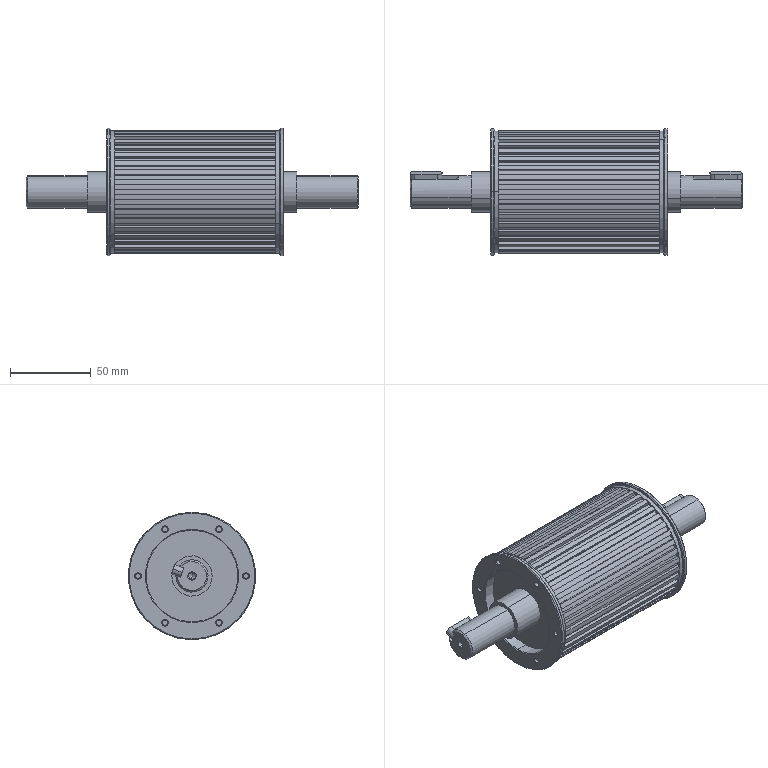Part | SolidWorks | 6 solids | 341 faces | box 206 x 79 x 79 mm | volume 296188 mm3 | cylinder 147 | plane 110 | cone 82 | spline 2 | commonest cylinder face diameters 76 x42 72 x39 3.2 x24 62 x12 6 x6 25 x6